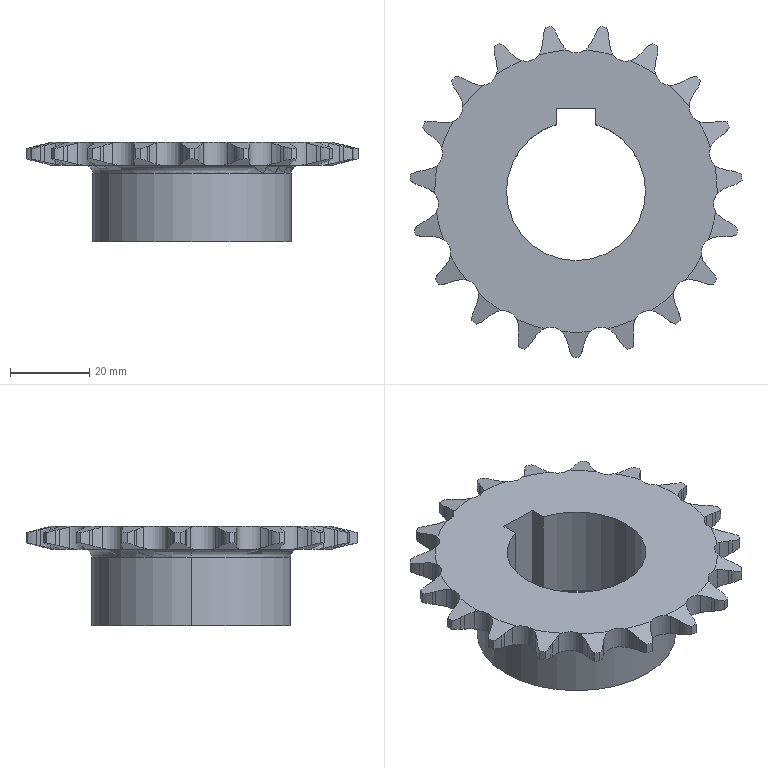Part | STEP file | 03-Small sprocket 1 | 1 solid | 208 faces | box 83.551 x 83.273 x 25 mm | volume 37685 mm3 | cylinder 119 | plane 44 | cone 43 | torus 2 | commonest cylinder face diameters 12.909 x38 20.25 x38 7.814 x19 83.727 x19 35 x3 50 x2